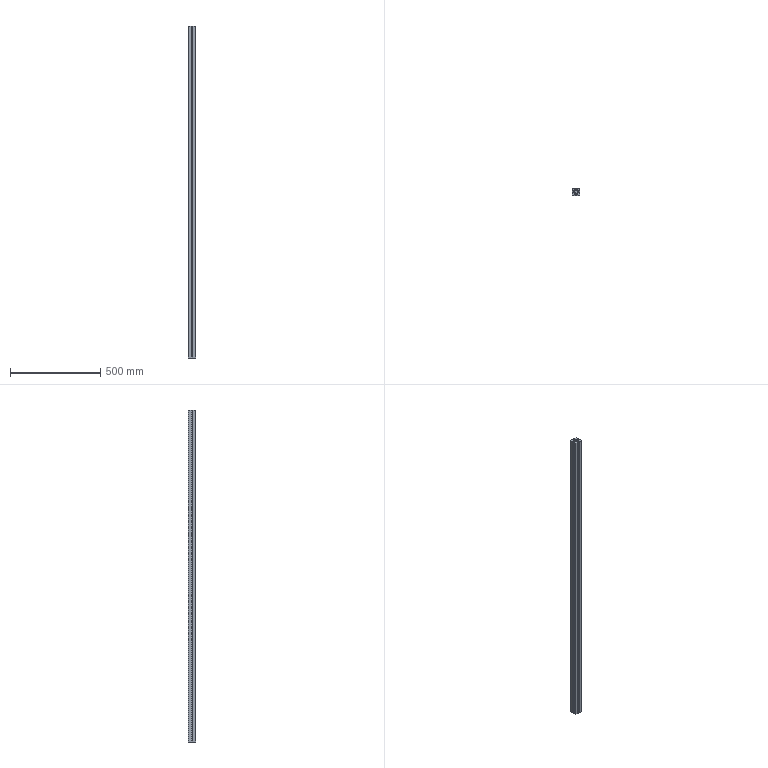Part | NX | 1 solid | 38 faces | box 40 x 40 x 1840 mm | volume 1840744 mm3 | plane 34 | cylinder 4 | commonest cylinder face diameters 19.333 x2 19.4 x2
STEP:
#1=CARTESIAN_POINT('',(-125.,655.75,0.));
#2=VERTEX_POINT('',#1);
#3=CARTESIAN_POINT('',(-121.5,655.75,0.));
#4=VERTEX_POINT('',#3);
#5=CARTESIAN_POINT('',(-125.,655.75,0.));
#6=DIRECTION('',(1.,0.,0.));
#7=VECTOR('',#6,1000.);
#8=LINE('',#5,#7);
#9=EDGE_CURVE('',#2,#4,#8,.T.);
#10=ORIENTED_EDGE('',*,*,#9,.T.);
#11=CARTESIAN_POINT('',(-121.5,655.75,-1840.));
#12=VERTEX_POINT('',#11);
#13=CARTESIAN_POINT('',(-121.5,655.75,-1840.));
#14=DIRECTION('',(0.,0.,1.));
#15=VECTOR('',#14,1000.);
#16=LINE('',#13,#15);
#17=EDGE_CURVE('',#12,#4,#16,.T.);
#18=ORIENTED_EDGE('',*,*,#17,.F.);
#19=CARTESIAN_POINT('',(-125.,655.75,-1840.));
#20=VERTEX_POINT('',#19);
#21=CARTESIAN_POINT('',(-125.,655.75,-1840.));
#22=DIRECTION('',(1.,0.,0.));
#23=VECTOR('',#22,1000.);
#24=LINE('',#21,#23);
#25=EDGE_CURVE('',#20,#12,#24,.T.);
#26=ORIENTED_EDGE('',*,*,#25,.F.);
#27=CARTESIAN_POINT('',(-125.,655.75,-1840.));
#28=DIRECTION('',(0.,0.,1.));
#29=VECTOR('',#28,1000.);
#30=LINE('',#27,#29);
#31=EDGE_CURVE('',#20,#2,#30,.T.);
#32=ORIENTED_EDGE('',*,*,#31,.T.);
#33=EDGE_LOOP('',(#10,#18,#26,#32));
#34=FACE_BOUND('',#33,.T.);
#35=CARTESIAN_POINT('',(-125.,655.75,-1840.));
#36=DIRECTION('',(0.,-1.,0.));
#37=DIRECTION('',(0.,0.,-1.));
#38=AXIS2_PLACEMENT_3D('',#35,#36,#37);
#39=PLANE('',#38);
#40=ADVANCED_FACE('',(#34),#39,.F.);
#41=CARTESIAN_POINT('',(-121.5,653.,0.));
#42=VERTEX_POINT('',#41);
#43=CARTESIAN_POINT('',(-121.5,655.75,0.));
#44=DIRECTION('',(0.,-1.,0.));
#45=VECTOR('',#44,1000.);
#46=LINE('',#43,#45);
#47=EDGE_CURVE('',#4,#42,#46,.T.);
#48=ORIENTED_EDGE('',*,*,#47,.T.);
#49=CARTESIAN_POINT('',(-121.5,653.,-1840.));
#50=VERTEX_POINT('',#49);
#51=CARTESIAN_POINT('',(-121.5,653.,-1840.));
#52=DIRECTION('',(0.,0.,1.));
#53=VECTOR('',#52,1000.);
#54=LINE('',#51,#53);
#55=EDGE_CURVE('',#50,#42,#54,.T.);
#56=ORIENTED_EDGE('',*,*,#55,.F.);
#57=CARTESIAN_POINT('',(-121.5,655.75,-1840.));
#58=DIRECTION('',(0.,-1.,0.));
#59=VECTOR('',#58,1000.);
#60=LINE('',#57,#59);
#61=EDGE_CURVE('',#12,#50,#60,.T.);
#62=ORIENTED_EDGE('',*,*,#61,.F.);
#63=ORIENTED_EDGE('',*,*,#17,.T.);
#64=EDGE_LOOP('',(#48,#56,#62,#63));
#65=FACE_BOUND('',#64,.T.);
#66=CARTESIAN_POINT('',(-121.5,655.75,-1840.));
#67=DIRECTION('',(-1.,0.,0.));
#68=DIRECTION('',(0.,0.,1.));
#69=AXIS2_PLACEMENT_3D('',#66,#67,#68);
#70=PLANE('',#69);
#71=ADVANCED_FACE('',(#65),#70,.F.);
#72=CARTESIAN_POINT('',(-114.5,653.,0.));
#73=VERTEX_POINT('',#72);
#74=CARTESIAN_POINT('',(-121.5,653.,0.));
#75=DIRECTION('',(1.,0.,0.));
#76=VECTOR('',#75,1000.);
#77=LINE('',#74,#76);
#78=EDGE_CURVE('',#42,#73,#77,.T.);
#79=ORIENTED_EDGE('',*,*,#78,.T.);
#80=CARTESIAN_POINT('',(-114.5,653.,-1840.));
#81=VERTEX_POINT('',#80);
#82=CARTESIAN_POINT('',(-114.5,653.,-1840.));
#83=DIRECTION('',(0.,0.,1.));
#84=VECTOR('',#83,1000.);
#85=LINE('',#82,#84);
#86=EDGE_CURVE('',#81,#73,#85,.T.);
#87=ORIENTED_EDGE('',*,*,#86,.F.);
#88=CARTESIAN_POINT('',(-121.5,653.,-1840.));
#89=DIRECTION('',(1.,0.,0.));
#90=VECTOR('',#89,1000.);
#91=LINE('',#88,#90);
#92=EDGE_CURVE('',#50,#81,#91,.T.);
#93=ORIENTED_EDGE('',*,*,#92,.F.);
#94=ORIENTED_EDGE('',*,*,#55,.T.);
#95=EDGE_LOOP('',(#79,#87,#93,#94));
#96=FACE_BOUND('',#95,.T.);
#97=CARTESIAN_POINT('',(-121.5,653.,-1840.));
#98=DIRECTION('',(0.,-1.,0.));
#99=DIRECTION('',(0.,0.,-1.));
#100=AXIS2_PLACEMENT_3D('',#97,#98,#99);
#101=PLANE('',#100);
#102=ADVANCED_FACE('',(#96),#101,.F.);
#103=CARTESIAN_POINT('',(-114.5,667.,0.));
#104=VERTEX_POINT('',#103);
#105=CARTESIAN_POINT('',(-121.167,660.,0.));
#106=DIRECTION('',(0.,0.,1.));
#107=DIRECTION('',(-1.,0.,0.));
#108=AXIS2_PLACEMENT_3D('',#105,#106,#107);
#109=CIRCLE('',#108,9.667);
#110=EDGE_CURVE('',#73,#104,#109,.T.);
#111=ORIENTED_EDGE('',*,*,#110,.T.);
#112=CARTESIAN_POINT('',(-114.5,667.,-1840.));
#113=VERTEX_POINT('',#112);
#114=CARTESIAN_POINT('',(-114.5,667.,-1840.));
#115=DIRECTION('',(0.,0.,1.));
#116=VECTOR('',#115,1000.);
#117=LINE('',#114,#116);
#118=EDGE_CURVE('',#113,#104,#117,.T.);
#119=ORIENTED_EDGE('',*,*,#118,.F.);
#120=CARTESIAN_POINT('',(-121.167,660.,-1840.));
#121=DIRECTION('',(0.,0.,1.));
#122=DIRECTION('',(-1.,0.,0.));
#123=AXIS2_PLACEMENT_3D('',#120,#121,#122);
#124=CIRCLE('',#123,9.667);
#125=EDGE_CURVE('',#81,#113,#124,.T.);
#126=ORIENTED_EDGE('',*,*,#125,.F.);
#127=ORIENTED_EDGE('',*,*,#86,.T.);
#128=EDGE_LOOP('',(#111,#119,#126,#127));
#129=FACE_BOUND('',#128,.T.);
#130=CARTESIAN_POINT('',(-121.167,660.,-1840.));
#131=DIRECTION('',(0.,0.,1.));
#132=DIRECTION('',(1.,0.,0.));
#133=AXIS2_PLACEMENT_3D('',#130,#131,#132);
#134=CYLINDRICAL_SURFACE('',#133,9.667);
#135=ADVANCED_FACE('',(#129),#134,.F.);
#136=CARTESIAN_POINT('',(-121.5,667.,0.));
#137=VERTEX_POINT('',#136);
#138=CARTESIAN_POINT('',(-114.5,667.,0.));
#139=DIRECTION('',(-1.,0.,0.));
#140=VECTOR('',#139,1000.);
#141=LINE('',#138,#140);
#142=EDGE_CURVE('',#104,#137,#141,.T.);
#143=ORIENTED_EDGE('',*,*,#142,.T.);
#144=CARTESIAN_POINT('',(-121.5,667.,-1840.));
#145=VERTEX_POINT('',#144);
#146=CARTESIAN_POINT('',(-121.5,667.,-1840.));
#147=DIRECTION('',(0.,0.,1.));
#148=VECTOR('',#147,1000.);
#149=LINE('',#146,#148);
#150=EDGE_CURVE('',#145,#137,#149,.T.);
#151=ORIENTED_EDGE('',*,*,#150,.F.);
#152=CARTESIAN_POINT('',(-114.5,667.,-1840.));
#153=DIRECTION('',(-1.,0.,0.));
#154=VECTOR('',#153,1000.);
#155=LINE('',#152,#154);
#156=EDGE_CURVE('',#113,#145,#155,.T.);
#157=ORIENTED_EDGE('',*,*,#156,.F.);
#158=ORIENTED_EDGE('',*,*,#118,.T.);
#159=EDGE_LOOP('',(#143,#151,#157,#158));
#160=FACE_BOUND('',#159,.T.);
#161=CARTESIAN_POINT('',(-114.5,667.,-1840.));
#162=DIRECTION('',(0.,1.,0.));
#163=DIRECTION('',(0.,0.,1.));
#164=AXIS2_PLACEMENT_3D('',#161,#162,#163);
#165=PLANE('',#164);
#166=ADVANCED_FACE('',(#160),#165,.F.);
#167=CARTESIAN_POINT('',(-121.5,664.25,0.));
#168=VERTEX_POINT('',#167);
#169=CARTESIAN_POINT('',(-121.5,667.,0.));
#170=DIRECTION('',(0.,-1.,0.));
#171=VECTOR('',#170,1000.);
#172=LINE('',#169,#171);
#173=EDGE_CURVE('',#137,#168,#172,.T.);
#174=ORIENTED_EDGE('',*,*,#173,.T.);
#175=CARTESIAN_POINT('',(-121.5,664.25,-1840.));
#176=VERTEX_POINT('',#175);
#177=CARTESIAN_POINT('',(-121.5,664.25,-1840.));
#178=DIRECTION('',(0.,0.,1.));
#179=VECTOR('',#178,1000.);
#180=LINE('',#177,#179);
#181=EDGE_CURVE('',#176,#168,#180,.T.);
#182=ORIENTED_EDGE('',*,*,#181,.F.);
#183=CARTESIAN_POINT('',(-121.5,667.,-1840.));
#184=DIRECTION('',(0.,-1.,0.));
#185=VECTOR('',#184,1000.);
#186=LINE('',#183,#185);
#187=EDGE_CURVE('',#145,#176,#186,.T.);
#188=ORIENTED_EDGE('',*,*,#187,.F.);
#189=ORIENTED_EDGE('',*,*,#150,.T.);
#190=EDGE_LOOP('',(#174,#182,#188,#189));
#191=FACE_BOUND('',#190,.T.);
#192=CARTESIAN_POINT('',(-121.5,667.,-1840.));
#193=DIRECTION('',(-1.,0.,0.));
#194=DIRECTION('',(0.,0.,1.));
#195=AXIS2_PLACEMENT_3D('',#192,#193,#194);
#196=PLANE('',#195);
#197=ADVANCED_FACE('',(#191),#196,.F.);
#198=CARTESIAN_POINT('',(-125.,664.25,0.));
#199=VERTEX_POINT('',#198);
#200=CARTESIAN_POINT('',(-121.5,664.25,0.));
#201=DIRECTION('',(-1.,0.,0.));
#202=VECTOR('',#201,1000.);
#203=LINE('',#200,#202);
#204=EDGE_CURVE('',#168,#199,#203,.T.);
#205=ORIENTED_EDGE('',*,*,#204,.T.);
#206=CARTESIAN_POINT('',(-125.,664.25,-1840.));
#207=VERTEX_POINT('',#206);
#208=CARTESIAN_POINT('',(-125.,664.25,-1840.));
#209=DIRECTION('',(0.,0.,1.));
#210=VECTOR('',#209,1000.);
#211=LINE('',#208,#210);
#212=EDGE_CURVE('',#207,#199,#211,.T.);
#213=ORIENTED_EDGE('',*,*,#212,.F.);
#214=CARTESIAN_POINT('',(-121.5,664.25,-1840.));
#215=DIRECTION('',(-1.,0.,0.));
#216=VECTOR('',#215,1000.);
#217=LINE('',#214,#216);
#218=EDGE_CURVE('',#176,#207,#217,.T.);
#219=ORIENTED_EDGE('',*,*,#218,.F.);
#220=ORIENTED_EDGE('',*,*,#181,.T.);
#221=EDGE_LOOP('',(#205,#213,#219,#220));
#222=FACE_BOUND('',#221,.T.);
#223=CARTESIAN_POINT('',(-121.5,664.25,-1840.));
#224=DIRECTION('',(0.,1.,0.));
#225=DIRECTION('',(0.,0.,1.));
#226=AXIS2_PLACEMENT_3D('',#223,#224,#225);
#227=PLANE('',#226);
#228=ADVANCED_FACE('',(#222),#227,.F.);
#229=CARTESIAN_POINT('',(-125.,680.,0.));
#230=VERTEX_POINT('',#229);
#231=CARTESIAN_POINT('',(-125.,680.,0.));
#232=DIRECTION('',(0.,1.,0.));
#233=VECTOR('',#232,1000.);
#234=LINE('',#231,#233);
#235=EDGE_CURVE('',#199,#230,#234,.T.);
#236=ORIENTED_EDGE('',*,*,#235,.T.);
#237=CARTESIAN_POINT('',(-125.,680.,-1840.));
#238=VERTEX_POINT('',#237);
#239=CARTESIAN_POINT('',(-125.,680.,-1840.));
#240=DIRECTION('',(0.,0.,1.));
#241=VECTOR('',#240,1000.);
#242=LINE('',#239,#241);
#243=EDGE_CURVE('',#238,#230,#242,.T.);
#244=ORIENTED_EDGE('',*,*,#243,.F.);
#245=CARTESIAN_POINT('',(-125.,664.25,-1840.));
#246=DIRECTION('',(0.,1.,0.));
#247=VECTOR('',#246,1000.);
#248=LINE('',#245,#247);
#249=EDGE_CURVE('',#207,#238,#248,.T.);
#250=ORIENTED_EDGE('',*,*,#249,.F.);
#251=ORIENTED_EDGE('',*,*,#212,.T.);
#252=EDGE_LOOP('',(#236,#244,#250,#251));
#253=FACE_BOUND('',#252,.T.);
#254=CARTESIAN_POINT('',(-125.,680.,-1840.));
#255=DIRECTION('',(1.,0.,0.));
#256=DIRECTION('',(0.,0.,-1.));
#257=AXIS2_PLACEMENT_3D('',#254,#255,#256);
#258=PLANE('',#257);
#259=ADVANCED_FACE('',(#253),#258,.F.);
#260=CARTESIAN_POINT('',(-109.25,680.,0.));
#261=VERTEX_POINT('',#260);
#262=CARTESIAN_POINT('',(-124.5,680.,0.));
#263=DIRECTION('',(1.,0.,0.));
#264=VECTOR('',#263,1000.);
#265=LINE('',#262,#264);
#266=EDGE_CURVE('',#230,#261,#265,.T.);
#267=ORIENTED_EDGE('',*,*,#266,.T.);
#268=CARTESIAN_POINT('',(-109.25,680.,-1840.));
#269=VERTEX_POINT('',#268);
#270=CARTESIAN_POINT('',(-109.25,680.,-1840.));
#271=DIRECTION('',(0.,0.,1.));
#272=VECTOR('',#271,1000.);
#273=LINE('',#270,#272);
#274=EDGE_CURVE('',#269,#261,#273,.T.);
#275=ORIENTED_EDGE('',*,*,#274,.F.);
#276=CARTESIAN_POINT('',(-124.5,680.,-1840.));
#277=DIRECTION('',(1.,0.,0.));
#278=VECTOR('',#277,1000.);
#279=LINE('',#276,#278);
#280=EDGE_CURVE('',#238,#269,#279,.T.);
#281=ORIENTED_EDGE('',*,*,#280,.F.);
#282=ORIENTED_EDGE('',*,*,#243,.T.);
#283=EDGE_LOOP('',(#267,#275,#281,#282));
#284=FACE_BOUND('',#283,.T.);
#285=CARTESIAN_POINT('',(-124.5,680.,-1840.));
#286=DIRECTION('',(0.,-1.,0.));
#287=DIRECTION('',(0.,0.,-1.));
#288=AXIS2_PLACEMENT_3D('',#285,#286,#287);
#289=PLANE('',#288);
#290=ADVANCED_FACE('',(#284),#289,.F.);
#291=CARTESIAN_POINT('',(-109.25,676.5,0.));
#292=VERTEX_POINT('',#291);
#293=CARTESIAN_POINT('',(-109.25,680.,0.));
#294=DIRECTION('',(0.,-1.,0.));
#295=VECTOR('',#294,1000.);
#296=LINE('',#293,#295);
#297=EDGE_CURVE('',#261,#292,#296,.T.);
#298=ORIENTED_EDGE('',*,*,#297,.T.);
#299=CARTESIAN_POINT('',(-109.25,676.5,-1840.));
#300=VERTEX_POINT('',#299);
#301=CARTESIAN_POINT('',(-109.25,676.5,-1840.));
#302=DIRECTION('',(0.,0.,1.));
#303=VECTOR('',#302,1000.);
#304=LINE('',#301,#303);
#305=EDGE_CURVE('',#300,#292,#304,.T.);
#306=ORIENTED_EDGE('',*,*,#305,.F.);
#307=CARTESIAN_POINT('',(-109.25,680.,-1840.));
#308=DIRECTION('',(0.,-1.,0.));
#309=VECTOR('',#308,1000.);
#310=LINE('',#307,#309);
#311=EDGE_CURVE('',#269,#300,#310,.T.);
#312=ORIENTED_EDGE('',*,*,#311,.F.);
#313=ORIENTED_EDGE('',*,*,#274,.T.);
#314=EDGE_LOOP('',(#298,#306,#312,#313));
#315=FACE_BOUND('',#314,.T.);
#316=CARTESIAN_POINT('',(-109.25,680.,-1840.));
#317=DIRECTION('',(-1.,0.,0.));
#318=DIRECTION('',(0.,0.,1.));
#319=AXIS2_PLACEMENT_3D('',#316,#317,#318);
#320=PLANE('',#319);
#321=ADVANCED_FACE('',(#315),#320,.F.);
#322=CARTESIAN_POINT('',(-111.5,676.5,0.));
#323=VERTEX_POINT('',#322);
#324=CARTESIAN_POINT('',(-109.25,676.5,0.));
#325=DIRECTION('',(-1.,0.,0.));
#326=VECTOR('',#325,1000.);
#327=LINE('',#324,#326);
#328=EDGE_CURVE('',#292,#323,#327,.T.);
#329=ORIENTED_EDGE('',*,*,#328,.T.);
#330=CARTESIAN_POINT('',(-111.5,676.5,-1840.));
#331=VERTEX_POINT('',#330);
#332=CARTESIAN_POINT('',(-111.5,676.5,-1840.));
#333=DIRECTION('',(0.,0.,1.));
#334=VECTOR('',#333,1000.);
#335=LINE('',#332,#334);
#336=EDGE_CURVE('',#331,#323,#335,.T.);
#337=ORIENTED_EDGE('',*,*,#336,.F.);
#338=CARTESIAN_POINT('',(-109.25,676.5,-1840.));
#339=DIRECTION('',(-1.,0.,0.));
#340=VECTOR('',#339,1000.);
#341=LINE('',#338,#340);
#342=EDGE_CURVE('',#300,#331,#341,.T.);
#343=ORIENTED_EDGE('',*,*,#342,.F.);
#344=ORIENTED_EDGE('',*,*,#305,.T.);
#345=EDGE_LOOP('',(#329,#337,#343,#344));
#346=FACE_BOUND('',#345,.T.);
#347=CARTESIAN_POINT('',(-109.25,676.5,-1840.));
#348=DIRECTION('',(0.,1.,0.));
#349=DIRECTION('',(0.,0.,1.));
#350=AXIS2_PLACEMENT_3D('',#347,#348,#349);
#351=PLANE('',#350);
#352=ADVANCED_FACE('',(#346),#351,.F.);
#353=CARTESIAN_POINT('',(-111.5,669.5,0.));
#354=VERTEX_POINT('',#353);
#355=CARTESIAN_POINT('',(-111.5,676.5,0.));
#356=DIRECTION('',(0.,-1.,0.));
#357=VECTOR('',#356,1000.);
#358=LINE('',#355,#357);
#359=EDGE_CURVE('',#323,#354,#358,.T.);
#360=ORIENTED_EDGE('',*,*,#359,.T.);
#361=CARTESIAN_POINT('',(-111.5,669.5,-1840.));
#362=VERTEX_POINT('',#361);
#363=CARTESIAN_POINT('',(-111.5,669.5,-1840.));
#364=DIRECTION('',(0.,0.,1.));
#365=VECTOR('',#364,1000.);
#366=LINE('',#363,#365);
#367=EDGE_CURVE('',#362,#354,#366,.T.);
#368=ORIENTED_EDGE('',*,*,#367,.F.);
#369=CARTESIAN_POINT('',(-111.5,676.5,-1840.));
#370=DIRECTION('',(0.,-1.,0.));
#371=VECTOR('',#370,1000.);
#372=LINE('',#369,#371);
#373=EDGE_CURVE('',#331,#362,#372,.T.);
#374=ORIENTED_EDGE('',*,*,#373,.F.);
#375=ORIENTED_EDGE('',*,*,#336,.T.);
#376=EDGE_LOOP('',(#360,#368,#374,#375));
#377=FACE_BOUND('',#376,.T.);
#378=CARTESIAN_POINT('',(-111.5,676.5,-1840.));
#379=DIRECTION('',(-1.,0.,0.));
#380=DIRECTION('',(0.,0.,1.));
#381=AXIS2_PLACEMENT_3D('',#378,#379,#380);
#382=PLANE('',#381);
#383=ADVANCED_FACE('',(#377),#382,.F.);
#384=CARTESIAN_POINT('',(-98.5,669.5,0.));
#385=VERTEX_POINT('',#384);
#386=CARTESIAN_POINT('',(-105.,676.7,0.));
#387=DIRECTION('',(0.,0.,1.));
#388=DIRECTION('',(-1.,0.,0.));
#389=AXIS2_PLACEMENT_3D('',#386,#387,#388);
#390=CIRCLE('',#389,9.7);
#391=EDGE_CURVE('',#354,#385,#390,.T.);
#392=ORIENTED_EDGE('',*,*,#391,.T.);
#393=CARTESIAN_POINT('',(-98.5,669.5,-1840.));
#394=VERTEX_POINT('',#393);
#395=CARTESIAN_POINT('',(-98.5,669.5,-1840.));
#396=DIRECTION('',(0.,0.,1.));
#397=VECTOR('',#396,1000.);
#398=LINE('',#395,#397);
#399=EDGE_CURVE('',#394,#385,#398,.T.);
#400=ORIENTED_EDGE('',*,*,#399,.F.);
#401=CARTESIAN_POINT('',(-105.,676.7,-1840.));
#402=DIRECTION('',(0.,0.,1.));
#403=DIRECTION('',(-1.,0.,0.));
#404=AXIS2_PLACEMENT_3D('',#401,#402,#403);
#405=CIRCLE('',#404,9.7);
#406=EDGE_CURVE('',#362,#394,#405,.T.);
#407=ORIENTED_EDGE('',*,*,#406,.F.);
#408=ORIENTED_EDGE('',*,*,#367,.T.);
#409=EDGE_LOOP('',(#392,#400,#407,#408));
#410=FACE_BOUND('',#409,.T.);
#411=CARTESIAN_POINT('',(-105.,676.7,-1840.));
#412=DIRECTION('',(0.,0.,1.));
#413=DIRECTION('',(1.,0.,0.));
#414=AXIS2_PLACEMENT_3D('',#411,#412,#413);
#415=CYLINDRICAL_SURFACE('',#414,9.7);
#416=ADVANCED_FACE('',(#410),#415,.F.);
#417=CARTESIAN_POINT('',(-98.5,676.5,0.));
#418=VERTEX_POINT('',#417);
#419=CARTESIAN_POINT('',(-98.5,669.5,0.));
#420=DIRECTION('',(0.,1.,0.));
#421=VECTOR('',#420,1000.);
#422=LINE('',#419,#421);
#423=EDGE_CURVE('',#385,#418,#422,.T.);
#424=ORIENTED_EDGE('',*,*,#423,.T.);
#425=CARTESIAN_POINT('',(-98.5,676.5,-1840.));
#426=VERTEX_POINT('',#425);
#427=CARTESIAN_POINT('',(-98.5,676.5,-1840.));
#428=DIRECTION('',(0.,0.,1.));
#429=VECTOR('',#428,1000.);
#430=LINE('',#427,#429);
#431=EDGE_CURVE('',#426,#418,#430,.T.);
#432=ORIENTED_EDGE('',*,*,#431,.F.);
#433=CARTESIAN_POINT('',(-98.5,669.5,-1840.));
#434=DIRECTION('',(0.,1.,0.));
#435=VECTOR('',#434,1000.);
#436=LINE('',#433,#435);
#437=EDGE_CURVE('',#394,#426,#436,.T.);
#438=ORIENTED_EDGE('',*,*,#437,.F.);
#439=ORIENTED_EDGE('',*,*,#399,.T.);
#440=EDGE_LOOP('',(#424,#432,#438,#439));
#441=FACE_BOUND('',#440,.T.);
#442=CARTESIAN_POINT('',(-98.5,669.5,-1840.));
#443=DIRECTION('',(1.,0.,0.));
#444=DIRECTION('',(0.,0.,-1.));
#445=AXIS2_PLACEMENT_3D('',#442,#443,#444);
#446=PLANE('',#445);
#447=ADVANCED_FACE('',(#441),#446,.F.);
#448=CARTESIAN_POINT('',(-100.75,676.5,0.));
#449=VERTEX_POINT('',#448);
#450=CARTESIAN_POINT('',(-98.5,676.5,0.));
#451=DIRECTION('',(-1.,0.,0.));
#452=VECTOR('',#451,1000.);
#453=LINE('',#450,#452);
#454=EDGE_CURVE('',#418,#449,#453,.T.);
#455=ORIENTED_EDGE('',*,*,#454,.T.);
#456=CARTESIAN_POINT('',(-100.75,676.5,-1840.));
#457=VERTEX_POINT('',#456);
#458=CARTESIAN_POINT('',(-100.75,676.5,-1840.));
#459=DIRECTION('',(0.,0.,1.));
#460=VECTOR('',#459,1000.);
#461=LINE('',#458,#460);
#462=EDGE_CURVE('',#457,#449,#461,.T.);
#463=ORIENTED_EDGE('',*,*,#462,.F.);
#464=CARTESIAN_POINT('',(-98.5,676.5,-1840.));
#465=DIRECTION('',(-1.,0.,0.));
#466=VECTOR('',#465,1000.);
#467=LINE('',#464,#466);
#468=EDGE_CURVE('',#426,#457,#467,.T.);
#469=ORIENTED_EDGE('',*,*,#468,.F.);
#470=ORIENTED_EDGE('',*,*,#431,.T.);
#471=EDGE_LOOP('',(#455,#463,#469,#470));
#472=FACE_BOUND('',#471,.T.);
#473=CARTESIAN_POINT('',(-98.5,676.5,-1840.));
#474=DIRECTION('',(0.,1.,0.));
#475=DIRECTION('',(0.,0.,1.));
#476=AXIS2_PLACEMENT_3D('',#473,#474,#475);
#477=PLANE('',#476);
#478=ADVANCED_FACE('',(#472),#477,.F.);
#479=CARTESIAN_POINT('',(-100.75,680.,0.));
#480=VERTEX_POINT('',#479);
#481=CARTESIAN_POINT('',(-100.75,676.5,0.));
#482=DIRECTION('',(0.,1.,0.));
#483=VECTOR('',#482,1000.);
#484=LINE('',#481,#483);
#485=EDGE_CURVE('',#449,#480,#484,.T.);
#486=ORIENTED_EDGE('',*,*,#485,.T.);
#487=CARTESIAN_POINT('',(-100.75,680.,-1840.));
#488=VERTEX_POINT('',#487);
#489=CARTESIAN_POINT('',(-100.75,680.,-1840.));
#490=DIRECTION('',(0.,0.,1.));
#491=VECTOR('',#490,1000.);
#492=LINE('',#489,#491);
#493=EDGE_CURVE('',#488,#480,#492,.T.);
#494=ORIENTED_EDGE('',*,*,#493,.F.);
#495=CARTESIAN_POINT('',(-100.75,676.5,-1840.));
#496=DIRECTION('',(0.,1.,0.));
#497=VECTOR('',#496,1000.);
#498=LINE('',#495,#497);
#499=EDGE_CURVE('',#457,#488,#498,.T.);
#500=ORIENTED_EDGE('',*,*,#499,.F.);
#501=ORIENTED_EDGE('',*,*,#462,.T.);
#502=EDGE_LOOP('',(#486,#494,#500,#501));
#503=FACE_BOUND('',#502,.T.);
#504=CARTESIAN_POINT('',(-100.75,676.5,-1840.));
#505=DIRECTION('',(1.,0.,0.));
#506=DIRECTION('',(0.,0.,-1.));
#507=AXIS2_PLACEMENT_3D('',#504,#505,#506);
#508=PLANE('',#507);
#509=ADVANCED_FACE('',(#503),#508,.F.);
#510=CARTESIAN_POINT('',(-85.,680.,0.));
#511=VERTEX_POINT('',#510);
#512=CARTESIAN_POINT('',(-85.5,680.,0.));
#513=DIRECTION('',(1.,0.,0.));
#514=VECTOR('',#513,1000.);
#515=LINE('',#512,#514);
#516=EDGE_CURVE('',#480,#511,#515,.T.);
#517=ORIENTED_EDGE('',*,*,#516,.T.);
#518=CARTESIAN_POINT('',(-85.,680.,-1840.));
#519=VERTEX_POINT('',#518);
#520=CARTESIAN_POINT('',(-85.,680.,-1840.));
#521=DIRECTION('',(0.,0.,1.));
#522=VECTOR('',#521,1000.);
#523=LINE('',#520,#522);
#524=EDGE_CURVE('',#519,#511,#523,.T.);
#525=ORIENTED_EDGE('',*,*,#524,.F.);
#526=CARTESIAN_POINT('',(-100.75,680.,-1840.));
#527=DIRECTION('',(1.,0.,0.));
#528=VECTOR('',#527,1000.);
#529=LINE('',#526,#528);
#530=EDGE_CURVE('',#488,#519,#529,.T.);
#531=ORIENTED_EDGE('',*,*,#530,.F.);
#532=ORIENTED_EDGE('',*,*,#493,.T.);
#533=EDGE_LOOP('',(#517,#525,#531,#532));
#534=FACE_BOUND('',#533,.T.);
#535=CARTESIAN_POINT('',(-85.5,680.,-1840.));
#536=DIRECTION('',(0.,-1.,0.));
#537=DIRECTION('',(0.,0.,-1.));
#538=AXIS2_PLACEMENT_3D('',#535,#536,#537);
#539=PLANE('',#538);
#540=ADVANCED_FACE('',(#534),#539,.F.);
#541=CARTESIAN_POINT('',(-85.,664.25,0.));
#542=VERTEX_POINT('',#541);
#543=CARTESIAN_POINT('',(-85.,679.5,0.));
#544=DIRECTION('',(0.,-1.,0.));
#545=VECTOR('',#544,1000.);
#546=LINE('',#543,#545);
#547=EDGE_CURVE('',#511,#542,#546,.T.);
#548=ORIENTED_EDGE('',*,*,#547,.T.);
#549=CARTESIAN_POINT('',(-85.,664.25,-1840.));
#550=VERTEX_POINT('',#549);
#551=CARTESIAN_POINT('',(-85.,664.25,-1840.));
#552=DIRECTION('',(0.,0.,1.));
#553=VECTOR('',#552,1000.);
#554=LINE('',#551,#553);
#555=EDGE_CURVE('',#550,#542,#554,.T.);
#556=ORIENTED_EDGE('',*,*,#555,.F.);
#557=CARTESIAN_POINT('',(-85.,680.,-1840.));
#558=DIRECTION('',(0.,-1.,0.));
#559=VECTOR('',#558,1000.);
#560=LINE('',#557,#559);
#561=EDGE_CURVE('',#519,#550,#560,.T.);
#562=ORIENTED_EDGE('',*,*,#561,.F.);
#563=ORIENTED_EDGE('',*,*,#524,.T.);
#564=EDGE_LOOP('',(#548,#556,#562,#563));
#565=FACE_BOUND('',#564,.T.);
#566=CARTESIAN_POINT('',(-85.,679.5,-1840.));
#567=DIRECTION('',(-1.,0.,0.));
#568=DIRECTION('',(0.,0.,1.));
#569=AXIS2_PLACEMENT_3D('',#566,#567,#568);
#570=PLANE('',#569);
#571=ADVANCED_FACE('',(#565),#570,.F.);
#572=CARTESIAN_POINT('',(-88.5,664.25,0.));
#573=VERTEX_POINT('',#572);
#574=CARTESIAN_POINT('',(-85.,664.25,0.));
#575=DIRECTION('',(-1.,0.,0.));
#576=VECTOR('',#575,1000.);
#577=LINE('',#574,#576);
#578=EDGE_CURVE('',#542,#573,#577,.T.);
#579=ORIENTED_EDGE('',*,*,#578,.T.);
#580=CARTESIAN_POINT('',(-88.5,664.25,-1840.));
#581=VERTEX_POINT('',#580);
#582=CARTESIAN_POINT('',(-88.5,664.25,-1840.));
#583=DIRECTION('',(0.,0.,1.));
#584=VECTOR('',#583,1000.);
#585=LINE('',#582,#584);
#586=EDGE_CURVE('',#581,#573,#585,.T.);
#587=ORIENTED_EDGE('',*,*,#586,.F.);
#588=CARTESIAN_POINT('',(-85.,664.25,-1840.));
#589=DIRECTION('',(-1.,0.,0.));
#590=VECTOR('',#589,1000.);
#591=LINE('',#588,#590);
#592=EDGE_CURVE('',#550,#581,#591,.T.);
#593=ORIENTED_EDGE('',*,*,#592,.F.);
#594=ORIENTED_EDGE('',*,*,#555,.T.);
#595=EDGE_LOOP('',(#579,#587,#593,#594));
#596=FACE_BOUND('',#595,.T.);
#597=CARTESIAN_POINT('',(-85.,664.25,-1840.));
#598=DIRECTION('',(0.,1.,0.));
#599=DIRECTION('',(0.,0.,1.));
#600=AXIS2_PLACEMENT_3D('',#597,#598,#599);
#601=PLANE('',#600);
#602=ADVANCED_FACE('',(#596),#601,.F.);
#603=CARTESIAN_POINT('',(-88.5,667.,0.));
#604=VERTEX_POINT('',#603);
#605=CARTESIAN_POINT('',(-88.5,664.25,0.));
#606=DIRECTION('',(0.,1.,0.));
#607=VECTOR('',#606,1000.);
#608=LINE('',#605,#607);
#609=EDGE_CURVE('',#573,#604,#608,.T.);
#610=ORIENTED_EDGE('',*,*,#609,.T.);
#611=CARTESIAN_POINT('',(-88.5,667.,-1840.));
#612=VERTEX_POINT('',#611);
#613=CARTESIAN_POINT('',(-88.5,667.,-1840.));
#614=DIRECTION('',(0.,0.,1.));
#615=VECTOR('',#614,1000.);
#616=LINE('',#613,#615);
#617=EDGE_CURVE('',#612,#604,#616,.T.);
#618=ORIENTED_EDGE('',*,*,#617,.F.);
#619=CARTESIAN_POINT('',(-88.5,664.25,-1840.));
#620=DIRECTION('',(0.,1.,0.));
#621=VECTOR('',#620,1000.);
#622=LINE('',#619,#621);
#623=EDGE_CURVE('',#581,#612,#622,.T.);
#624=ORIENTED_EDGE('',*,*,#623,.F.);
#625=ORIENTED_EDGE('',*,*,#586,.T.);
#626=EDGE_LOOP('',(#610,#618,#624,#625));
#627=FACE_BOUND('',#626,.T.);
#628=CARTESIAN_POINT('',(-88.5,664.25,-1840.));
#629=DIRECTION('',(1.,0.,0.));
#630=DIRECTION('',(0.,0.,-1.));
#631=AXIS2_PLACEMENT_3D('',#628,#629,#630);
#632=PLANE('',#631);
#633=ADVANCED_FACE('',(#627),#632,.F.);
#634=CARTESIAN_POINT('',(-95.5,667.,0.));
#635=VERTEX_POINT('',#634);
#636=CARTESIAN_POINT('',(-88.5,667.,0.));
#637=DIRECTION('',(-1.,0.,0.));
#638=VECTOR('',#637,1000.);
#639=LINE('',#636,#638);
#640=EDGE_CURVE('',#604,#635,#639,.T.);
#641=ORIENTED_EDGE('',*,*,#640,.T.);
#642=CARTESIAN_POINT('',(-95.5,667.,-1840.));
#643=VERTEX_POINT('',#642);
#644=CARTESIAN_POINT('',(-95.5,667.,-1840.));
#645=DIRECTION('',(0.,0.,1.));
#646=VECTOR('',#645,1000.);
#647=LINE('',#644,#646);
#648=EDGE_CURVE('',#643,#635,#647,.T.);
#649=ORIENTED_EDGE('',*,*,#648,.F.);
#650=CARTESIAN_POINT('',(-88.5,667.,-1840.));
#651=DIRECTION('',(-1.,0.,0.));
#652=VECTOR('',#651,1000.);
#653=LINE('',#650,#652);
#654=EDGE_CURVE('',#612,#643,#653,.T.);
#655=ORIENTED_EDGE('',*,*,#654,.F.);
#656=ORIENTED_EDGE('',*,*,#617,.T.);
#657=EDGE_LOOP('',(#641,#649,#655,#656));
#658=FACE_BOUND('',#657,.T.);
#659=CARTESIAN_POINT('',(-88.5,667.,-1840.));
#660=DIRECTION('',(0.,1.,0.));
#661=DIRECTION('',(0.,0.,1.));
#662=AXIS2_PLACEMENT_3D('',#659,#660,#661);
#663=PLANE('',#662);
#664=ADVANCED_FACE('',(#658),#663,.F.);
#665=CARTESIAN_POINT('',(-95.5,653.,0.));
#666=VERTEX_POINT('',#665);
#667=CARTESIAN_POINT('',(-88.833,660.,0.));
#668=DIRECTION('',(0.,0.,1.));
#669=DIRECTION('',(-1.,0.,0.));
#670=AXIS2_PLACEMENT_3D('',#667,#668,#669);
#671=CIRCLE('',#670,9.667);
#672=EDGE_CURVE('',#635,#666,#671,.T.);
#673=ORIENTED_EDGE('',*,*,#672,.T.);
#674=CARTESIAN_POINT('',(-95.5,653.,-1840.));
#675=VERTEX_POINT('',#674);
#676=CARTESIAN_POINT('',(-95.5,653.,-1840.));
#677=DIRECTION('',(0.,0.,1.));
#678=VECTOR('',#677,1000.);
#679=LINE('',#676,#678);
#680=EDGE_CURVE('',#675,#666,#679,.T.);
#681=ORIENTED_EDGE('',*,*,#680,.F.);
#682=CARTESIAN_POINT('',(-88.833,660.,-1840.));
#683=DIRECTION('',(0.,0.,1.));
#684=DIRECTION('',(-1.,0.,0.));
#685=AXIS2_PLACEMENT_3D('',#682,#683,#684);
#686=CIRCLE('',#685,9.667);
#687=EDGE_CURVE('',#643,#675,#686,.T.);
#688=ORIENTED_EDGE('',*,*,#687,.F.);
#689=ORIENTED_EDGE('',*,*,#648,.T.);
#690=EDGE_LOOP('',(#673,#681,#688,#689));
#691=FACE_BOUND('',#690,.T.);
#692=CARTESIAN_POINT('',(-88.833,660.,-1840.));
#693=DIRECTION('',(0.,0.,1.));
#694=DIRECTION('',(1.,0.,0.));
#695=AXIS2_PLACEMENT_3D('',#692,#693,#694);
#696=CYLINDRICAL_SURFACE('',#695,9.667);
#697=ADVANCED_FACE('',(#691),#696,.F.);
#698=CARTESIAN_POINT('',(-88.5,653.,0.));
#699=VERTEX_POINT('',#698);
#700=CARTESIAN_POINT('',(-95.5,653.,0.));
#701=DIRECTION('',(1.,0.,0.));
#702=VECTOR('',#701,1000.);
#703=LINE('',#700,#702);
#704=EDGE_CURVE('',#666,#699,#703,.T.);
#705=ORIENTED_EDGE('',*,*,#704,.T.);
#706=CARTESIAN_POINT('',(-88.5,653.,-1840.));
#707=VERTEX_POINT('',#706);
#708=CARTESIAN_POINT('',(-88.5,653.,-1840.));
#709=DIRECTION('',(0.,0.,1.));
#710=VECTOR('',#709,1000.);
#711=LINE('',#708,#710);
#712=EDGE_CURVE('',#707,#699,#711,.T.);
#713=ORIENTED_EDGE('',*,*,#712,.F.);
#714=CARTESIAN_POINT('',(-95.5,653.,-1840.));
#715=DIRECTION('',(1.,0.,0.));
#716=VECTOR('',#715,1000.);
#717=LINE('',#714,#716);
#718=EDGE_CURVE('',#675,#707,#717,.T.);
#719=ORIENTED_EDGE('',*,*,#718,.F.);
#720=ORIENTED_EDGE('',*,*,#680,.T.);
#721=EDGE_LOOP('',(#705,#713,#719,#720));
#722=FACE_BOUND('',#721,.T.);
#723=CARTESIAN_POINT('',(-95.5,653.,-1840.));
#724=DIRECTION('',(0.,-1.,0.));
#725=DIRECTION('',(0.,0.,-1.));
#726=AXIS2_PLACEMENT_3D('',#723,#724,#725);
#727=PLANE('',#726);
#728=ADVANCED_FACE('',(#722),#727,.F.);
#729=CARTESIAN_POINT('',(-88.5,655.75,0.));
#730=VERTEX_POINT('',#729);
#731=CARTESIAN_POINT('',(-88.5,653.,0.));
#732=DIRECTION('',(0.,1.,0.));
#733=VECTOR('',#732,1000.);
#734=LINE('',#731,#733);
#735=EDGE_CURVE('',#699,#730,#734,.T.);
#736=ORIENTED_EDGE('',*,*,#735,.T.);
#737=CARTESIAN_POINT('',(-88.5,655.75,-1840.));
#738=VERTEX_POINT('',#737);
#739=CARTESIAN_POINT('',(-88.5,655.75,-1840.));
#740=DIRECTION('',(0.,0.,1.));
#741=VECTOR('',#740,1000.);
#742=LINE('',#739,#741);
#743=EDGE_CURVE('',#738,#730,#742,.T.);
#744=ORIENTED_EDGE('',*,*,#743,.F.);
#745=CARTESIAN_POINT('',(-88.5,653.,-1840.));
#746=DIRECTION('',(0.,1.,0.));
#747=VECTOR('',#746,1000.);
#748=LINE('',#745,#747);
#749=EDGE_CURVE('',#707,#738,#748,.T.);
#750=ORIENTED_EDGE('',*,*,#749,.F.);
#751=ORIENTED_EDGE('',*,*,#712,.T.);
#752=EDGE_LOOP('',(#736,#744,#750,#751));
#753=FACE_BOUND('',#752,.T.);
#754=CARTESIAN_POINT('',(-88.5,653.,-1840.));
#755=DIRECTION('',(1.,0.,0.));
#756=DIRECTION('',(0.,0.,-1.));
#757=AXIS2_PLACEMENT_3D('',#754,#755,#756);
#758=PLANE('',#757);
#759=ADVANCED_FACE('',(#753),#758,.F.);
#760=CARTESIAN_POINT('',(-85.,655.75,0.));
#761=VERTEX_POINT('',#760);
#762=CARTESIAN_POINT('',(-88.5,655.75,0.));
#763=DIRECTION('',(1.,0.,0.));
#764=VECTOR('',#763,1000.);
#765=LINE('',#762,#764);
#766=EDGE_CURVE('',#730,#761,#765,.T.);
#767=ORIENTED_EDGE('',*,*,#766,.T.);
#768=CARTESIAN_POINT('',(-85.,655.75,-1840.));
#769=VERTEX_POINT('',#768);
#770=CARTESIAN_POINT('',(-85.,655.75,-1840.));
#771=DIRECTION('',(0.,0.,1.));
#772=VECTOR('',#771,1000.);
#773=LINE('',#770,#772);
#774=EDGE_CURVE('',#769,#761,#773,.T.);
#775=ORIENTED_EDGE('',*,*,#774,.F.);
#776=CARTESIAN_POINT('',(-88.5,655.75,-1840.));
#777=DIRECTION('',(1.,0.,0.));
#778=VECTOR('',#777,1000.);
#779=LINE('',#776,#778);
#780=EDGE_CURVE('',#738,#769,#779,.T.);
#781=ORIENTED_EDGE('',*,*,#780,.F.);
#782=ORIENTED_EDGE('',*,*,#743,.T.);
#783=EDGE_LOOP('',(#767,#775,#781,#782));
#784=FACE_BOUND('',#783,.T.);
#785=CARTESIAN_POINT('',(-88.5,655.75,-1840.));
#786=DIRECTION('',(0.,-1.,0.));
#787=DIRECTION('',(0.,0.,-1.));
#788=AXIS2_PLACEMENT_3D('',#785,#786,#787);
#789=PLANE('',#788);
#790=ADVANCED_FACE('',(#784),#789,.F.);
#791=CARTESIAN_POINT('',(-85.,640.,0.));
#792=VERTEX_POINT('',#791);
#793=CARTESIAN_POINT('',(-85.,640.5,0.));
#794=DIRECTION('',(0.,-1.,0.));
#795=VECTOR('',#794,1000.);
#796=LINE('',#793,#795);
#797=EDGE_CURVE('',#761,#792,#796,.T.);
#798=ORIENTED_EDGE('',*,*,#797,.T.);
#799=CARTESIAN_POINT('',(-85.,640.,-1840.));
#800=VERTEX_POINT('',#799);
#801=CARTESIAN_POINT('',(-85.,640.,-1840.));
#802=DIRECTION('',(0.,0.,1.));
#803=VECTOR('',#802,1000.);
#804=LINE('',#801,#803);
#805=EDGE_CURVE('',#800,#792,#804,.T.);
#806=ORIENTED_EDGE('',*,*,#805,.F.);
#807=CARTESIAN_POINT('',(-85.,655.75,-1840.));
#808=DIRECTION('',(0.,-1.,0.));
#809=VECTOR('',#808,1000.);
#810=LINE('',#807,#809);
#811=EDGE_CURVE('',#769,#800,#810,.T.);
#812=ORIENTED_EDGE('',*,*,#811,.F.);
#813=ORIENTED_EDGE('',*,*,#774,.T.);
#814=EDGE_LOOP('',(#798,#806,#812,#813));
#815=FACE_BOUND('',#814,.T.);
#816=CARTESIAN_POINT('',(-85.,640.5,-1840.));
#817=DIRECTION('',(-1.,0.,0.));
#818=DIRECTION('',(0.,0.,1.));
#819=AXIS2_PLACEMENT_3D('',#816,#817,#818);
#820=PLANE('',#819);
#821=ADVANCED_FACE('',(#815),#820,.F.);
#822=CARTESIAN_POINT('',(-100.75,640.,0.));
#823=VERTEX_POINT('',#822);
#824=CARTESIAN_POINT('',(-85.5,640.,0.));
#825=DIRECTION('',(-1.,0.,0.));
#826=VECTOR('',#825,1000.);
#827=LINE('',#824,#826);
#828=EDGE_CURVE('',#792,#823,#827,.T.);
#829=ORIENTED_EDGE('',*,*,#828,.T.);
#830=CARTESIAN_POINT('',(-100.75,640.,-1840.));
#831=VERTEX_POINT('',#830);
#832=CARTESIAN_POINT('',(-100.75,640.,-1840.));
#833=DIRECTION('',(0.,0.,1.));
#834=VECTOR('',#833,1000.);
#835=LINE('',#832,#834);
#836=EDGE_CURVE('',#831,#823,#835,.T.);
#837=ORIENTED_EDGE('',*,*,#836,.F.);
#838=CARTESIAN_POINT('',(-85.,640.,-1840.));
#839=DIRECTION('',(-1.,0.,0.));
#840=VECTOR('',#839,1000.);
#841=LINE('',#838,#840);
#842=EDGE_CURVE('',#800,#831,#841,.T.);
#843=ORIENTED_EDGE('',*,*,#842,.F.);
#844=ORIENTED_EDGE('',*,*,#805,.T.);
#845=EDGE_LOOP('',(#829,#837,#843,#844));
#846=FACE_BOUND('',#845,.T.);
#847=CARTESIAN_POINT('',(-85.5,640.,-1840.));
#848=DIRECTION('',(0.,1.,0.));
#849=DIRECTION('',(-1.,0.,0.));
#850=AXIS2_PLACEMENT_3D('',#847,#848,#849);
#851=PLANE('',#850);
#852=ADVANCED_FACE('',(#846),#851,.F.);
#853=CARTESIAN_POINT('',(-100.75,643.5,0.));
#854=VERTEX_POINT('',#853);
#855=CARTESIAN_POINT('',(-100.75,640.,0.));
#856=DIRECTION('',(0.,1.,0.));
#857=VECTOR('',#856,1000.);
#858=LINE('',#855,#857);
#859=EDGE_CURVE('',#823,#854,#858,.T.);
#860=ORIENTED_EDGE('',*,*,#859,.T.);
#861=CARTESIAN_POINT('',(-100.75,643.5,-1840.));
#862=VERTEX_POINT('',#861);
#863=CARTESIAN_POINT('',(-100.75,643.5,-1840.));
#864=DIRECTION('',(0.,0.,1.));
#865=VECTOR('',#864,1000.);
#866=LINE('',#863,#865);
#867=EDGE_CURVE('',#862,#854,#866,.T.);
#868=ORIENTED_EDGE('',*,*,#867,.F.);
#869=CARTESIAN_POINT('',(-100.75,640.,-1840.));
#870=DIRECTION('',(0.,1.,0.));
#871=VECTOR('',#870,1000.);
#872=LINE('',#869,#871);
#873=EDGE_CURVE('',#831,#862,#872,.T.);
#874=ORIENTED_EDGE('',*,*,#873,.F.);
#875=ORIENTED_EDGE('',*,*,#836,.T.);
#876=EDGE_LOOP('',(#860,#868,#874,#875));
#877=FACE_BOUND('',#876,.T.);
#878=CARTESIAN_POINT('',(-100.75,640.,-1840.));
#879=DIRECTION('',(1.,0.,0.));
#880=DIRECTION('',(0.,0.,-1.));
#881=AXIS2_PLACEMENT_3D('',#878,#879,#880);
#882=PLANE('',#881);
#883=ADVANCED_FACE('',(#877),#882,.F.);
#884=CARTESIAN_POINT('',(-98.5,643.5,0.));
#885=VERTEX_POINT('',#884);
#886=CARTESIAN_POINT('',(-100.75,643.5,0.));
#887=DIRECTION('',(1.,0.,0.));
#888=VECTOR('',#887,1000.);
#889=LINE('',#886,#888);
#890=EDGE_CURVE('',#854,#885,#889,.T.);
#891=ORIENTED_EDGE('',*,*,#890,.T.);
#892=CARTESIAN_POINT('',(-98.5,643.5,-1840.));
#893=VERTEX_POINT('',#892);
#894=CARTESIAN_POINT('',(-98.5,643.5,-1840.));
#895=DIRECTION('',(0.,0.,1.));
#896=VECTOR('',#895,1000.);
#897=LINE('',#894,#896);
#898=EDGE_CURVE('',#893,#885,#897,.T.);
#899=ORIENTED_EDGE('',*,*,#898,.F.);
#900=CARTESIAN_POINT('',(-100.75,643.5,-1840.));
#901=DIRECTION('',(1.,0.,0.));
#902=VECTOR('',#901,1000.);
#903=LINE('',#900,#902);
#904=EDGE_CURVE('',#862,#893,#903,.T.);
#905=ORIENTED_EDGE('',*,*,#904,.F.);
#906=ORIENTED_EDGE('',*,*,#867,.T.);
#907=EDGE_LOOP('',(#891,#899,#905,#906));
#908=FACE_BOUND('',#907,.T.);
#909=CARTESIAN_POINT('',(-100.75,643.5,-1840.));
#910=DIRECTION('',(0.,-1.,0.));
#911=DIRECTION('',(0.,0.,-1.));
#912=AXIS2_PLACEMENT_3D('',#909,#910,#911);
#913=PLANE('',#912);
#914=ADVANCED_FACE('',(#908),#913,.F.);
#915=CARTESIAN_POINT('',(-98.5,650.5,0.));
#916=VERTEX_POINT('',#915);
#917=CARTESIAN_POINT('',(-98.5,643.5,0.));
#918=DIRECTION('',(0.,1.,0.));
#919=VECTOR('',#918,1000.);
#920=LINE('',#917,#919);
#921=EDGE_CURVE('',#885,#916,#920,.T.);
#922=ORIENTED_EDGE('',*,*,#921,.T.);
#923=CARTESIAN_POINT('',(-98.5,650.5,-1840.));
#924=VERTEX_POINT('',#923);
#925=CARTESIAN_POINT('',(-98.5,650.5,-1840.));
#926=DIRECTION('',(0.,0.,1.));
#927=VECTOR('',#926,1000.);
#928=LINE('',#925,#927);
#929=EDGE_CURVE('',#924,#916,#928,.T.);
#930=ORIENTED_EDGE('',*,*,#929,.F.);
#931=CARTESIAN_POINT('',(-98.5,643.5,-1840.));
#932=DIRECTION('',(0.,1.,0.));
#933=VECTOR('',#932,1000.);
#934=LINE('',#931,#933);
#935=EDGE_CURVE('',#893,#924,#934,.T.);
#936=ORIENTED_EDGE('',*,*,#935,.F.);
#937=ORIENTED_EDGE('',*,*,#898,.T.);
#938=EDGE_LOOP('',(#922,#930,#936,#937));
#939=FACE_BOUND('',#938,.T.);
#940=CARTESIAN_POINT('',(-98.5,643.5,-1840.));
#941=DIRECTION('',(1.,0.,0.));
#942=DIRECTION('',(0.,1.,0.));
#943=AXIS2_PLACEMENT_3D('',#940,#941,#942);
#944=PLANE('',#943);
#945=ADVANCED_FACE('',(#939),#944,.F.);
#946=CARTESIAN_POINT('',(-111.5,650.5,0.));
#947=VERTEX_POINT('',#946);
#948=CARTESIAN_POINT('',(-105.,643.3,0.));
#949=DIRECTION('',(0.,0.,1.));
#950=DIRECTION('',(-1.,0.,0.));
#951=AXIS2_PLACEMENT_3D('',#948,#949,#950);
#952=CIRCLE('',#951,9.7);
#953=EDGE_CURVE('',#916,#947,#952,.T.);
#954=ORIENTED_EDGE('',*,*,#953,.T.);
#955=CARTESIAN_POINT('',(-111.5,650.5,-1840.));
#956=VERTEX_POINT('',#955);
#957=CARTESIAN_POINT('',(-111.5,650.5,-1840.));
#958=DIRECTION('',(0.,0.,1.));
#959=VECTOR('',#958,1000.);
#960=LINE('',#957,#959);
#961=EDGE_CURVE('',#956,#947,#960,.T.);
#962=ORIENTED_EDGE('',*,*,#961,.F.);
#963=CARTESIAN_POINT('',(-105.,643.3,-1840.));
#964=DIRECTION('',(0.,0.,1.));
#965=DIRECTION('',(-1.,0.,0.));
#966=AXIS2_PLACEMENT_3D('',#963,#964,#965);
#967=CIRCLE('',#966,9.7);
#968=EDGE_CURVE('',#924,#956,#967,.T.);
#969=ORIENTED_EDGE('',*,*,#968,.F.);
#970=ORIENTED_EDGE('',*,*,#929,.T.);
#971=EDGE_LOOP('',(#954,#962,#969,#970));
#972=FACE_BOUND('',#971,.T.);
#973=CARTESIAN_POINT('',(-105.,643.3,-1840.));
#974=DIRECTION('',(0.,0.,1.));
#975=DIRECTION('',(1.,0.,0.));
#976=AXIS2_PLACEMENT_3D('',#973,#974,#975);
#977=CYLINDRICAL_SURFACE('',#976,9.7);
#978=ADVANCED_FACE('',(#972),#977,.F.);
#979=CARTESIAN_POINT('',(-111.5,643.5,0.));
#980=VERTEX_POINT('',#979);
#981=CARTESIAN_POINT('',(-111.5,650.5,0.));
#982=DIRECTION('',(0.,-1.,0.));
#983=VECTOR('',#982,1000.);
#984=LINE('',#981,#983);
#985=EDGE_CURVE('',#947,#980,#984,.T.);
#986=ORIENTED_EDGE('',*,*,#985,.T.);
#987=CARTESIAN_POINT('',(-111.5,643.5,-1840.));
#988=VERTEX_POINT('',#987);
#989=CARTESIAN_POINT('',(-111.5,643.5,-1840.));
#990=DIRECTION('',(0.,0.,1.));
#991=VECTOR('',#990,1000.);
#992=LINE('',#989,#991);
#993=EDGE_CURVE('',#988,#980,#992,.T.);
#994=ORIENTED_EDGE('',*,*,#993,.F.);
#995=CARTESIAN_POINT('',(-111.5,650.5,-1840.));
#996=DIRECTION('',(0.,-1.,0.));
#997=VECTOR('',#996,1000.);
#998=LINE('',#995,#997);
#999=EDGE_CURVE('',#956,#988,#998,.T.);
#1000=ORIENTED_EDGE('',*,*,#999,.F.);
#1001=ORIENTED_EDGE('',*,*,#961,.T.);
#1002=EDGE_LOOP('',(#986,#994,#1000,#1001));
#1003=FACE_BOUND('',#1002,.T.);
#1004=CARTESIAN_POINT('',(-111.5,650.5,-1840.));
#1005=DIRECTION('',(-1.,0.,0.));
#1006=DIRECTION('',(0.,-1.,0.));
#1007=AXIS2_PLACEMENT_3D('',#1004,#1005,#1006);
#1008=PLANE('',#1007);
#1009=ADVANCED_FACE('',(#1003),#1008,.F.);
#1010=CARTESIAN_POINT('',(-109.25,643.5,0.));
#1011=VERTEX_POINT('',#1010);
#1012=CARTESIAN_POINT('',(-111.5,643.5,0.));
#1013=DIRECTION('',(1.,0.,0.));
#1014=VECTOR('',#1013,1000.);
#1015=LINE('',#1012,#1014);
#1016=EDGE_CURVE('',#980,#1011,#1015,.T.);
#1017=ORIENTED_EDGE('',*,*,#1016,.T.);
#1018=CARTESIAN_POINT('',(-109.25,643.5,-1840.));
#1019=VERTEX_POINT('',#1018);
#1020=CARTESIAN_POINT('',(-109.25,643.5,-1840.));
#1021=DIRECTION('',(0.,0.,1.));
#1022=VECTOR('',#1021,1000.);
#1023=LINE('',#1020,#1022);
#1024=EDGE_CURVE('',#1019,#1011,#1023,.T.);
#1025=ORIENTED_EDGE('',*,*,#1024,.F.);
#1026=CARTESIAN_POINT('',(-111.5,643.5,-1840.));
#1027=DIRECTION('',(1.,0.,0.));
#1028=VECTOR('',#1027,1000.);
#1029=LINE('',#1026,#1028);
#1030=EDGE_CURVE('',#988,#1019,#1029,.T.);
#1031=ORIENTED_EDGE('',*,*,#1030,.F.);
#1032=ORIENTED_EDGE('',*,*,#993,.T.);
#1033=EDGE_LOOP('',(#1017,#1025,#1031,#1032));
#1034=FACE_BOUND('',#1033,.T.);
#1035=CARTESIAN_POINT('',(-111.5,643.5,-1840.));
#1036=DIRECTION('',(0.,-1.,0.));
#1037=DIRECTION('',(0.,0.,-1.));
#1038=AXIS2_PLACEMENT_3D('',#1035,#1036,#1037);
#1039=PLANE('',#1038);
#1040=ADVANCED_FACE('',(#1034),#1039,.F.);
#1041=CARTESIAN_POINT('',(-109.25,640.,0.));
#1042=VERTEX_POINT('',#1041);
#1043=CARTESIAN_POINT('',(-109.25,643.5,0.));
#1044=DIRECTION('',(0.,-1.,0.));
#1045=VECTOR('',#1044,1000.);
#1046=LINE('',#1043,#1045);
#1047=EDGE_CURVE('',#1011,#1042,#1046,.T.);
#1048=ORIENTED_EDGE('',*,*,#1047,.T.);
#1049=CARTESIAN_POINT('',(-109.25,640.,-1840.));
#1050=VERTEX_POINT('',#1049);
#1051=CARTESIAN_POINT('',(-109.25,640.,-1840.));
#1052=DIRECTION('',(0.,0.,1.));
#1053=VECTOR('',#1052,1000.);
#1054=LINE('',#1051,#1053);
#1055=EDGE_CURVE('',#1050,#1042,#1054,.T.);
#1056=ORIENTED_EDGE('',*,*,#1055,.F.);
#1057=CARTESIAN_POINT('',(-109.25,643.5,-1840.));
#1058=DIRECTION('',(0.,-1.,0.));
#1059=VECTOR('',#1058,1000.);
#1060=LINE('',#1057,#1059);
#1061=EDGE_CURVE('',#1019,#1050,#1060,.T.);
#1062=ORIENTED_EDGE('',*,*,#1061,.F.);
#1063=ORIENTED_EDGE('',*,*,#1024,.T.);
#1064=EDGE_LOOP('',(#1048,#1056,#1062,#1063));
#1065=FACE_BOUND('',#1064,.T.);
#1066=CARTESIAN_POINT('',(-109.25,643.5,-1840.));
#1067=DIRECTION('',(-1.,0.,0.));
#1068=DIRECTION('',(0.,0.,1.));
#1069=AXIS2_PLACEMENT_3D('',#1066,#1067,#1068);
#1070=PLANE('',#1069);
#1071=ADVANCED_FACE('',(#1065),#1070,.F.);
#1072=CARTESIAN_POINT('',(-125.,640.,0.));
#1073=VERTEX_POINT('',#1072);
#1074=CARTESIAN_POINT('',(-125.,640.,0.));
#1075=DIRECTION('',(-1.,0.,0.));
#1076=VECTOR('',#1075,1000.);
#1077=LINE('',#1074,#1076);
#1078=EDGE_CURVE('',#1042,#1073,#1077,.T.);
#1079=ORIENTED_EDGE('',*,*,#1078,.T.);
#1080=CARTESIAN_POINT('',(-125.,640.,-1840.));
#1081=VERTEX_POINT('',#1080);
#1082=CARTESIAN_POINT('',(-125.,640.,-1840.));
#1083=DIRECTION('',(0.,0.,1.));
#1084=VECTOR('',#1083,1000.);
#1085=LINE('',#1082,#1084);
#1086=EDGE_CURVE('',#1081,#1073,#1085,.T.);
#1087=ORIENTED_EDGE('',*,*,#1086,.F.);
#1088=CARTESIAN_POINT('',(-109.25,640.,-1840.));
#1089=DIRECTION('',(-1.,0.,0.));
#1090=VECTOR('',#1089,1000.);
#1091=LINE('',#1088,#1090);
#1092=EDGE_CURVE('',#1050,#1081,#1091,.T.);
#1093=ORIENTED_EDGE('',*,*,#1092,.F.);
#1094=ORIENTED_EDGE('',*,*,#1055,.T.);
#1095=EDGE_LOOP('',(#1079,#1087,#1093,#1094));
#1096=FACE_BOUND('',#1095,.T.);
#1097=CARTESIAN_POINT('',(-125.,640.,-1840.));
#1098=DIRECTION('',(0.,1.,0.));
#1099=DIRECTION('',(0.,0.,1.));
#1100=AXIS2_PLACEMENT_3D('',#1097,#1098,#1099);
#1101=PLANE('',#1100);
#1102=ADVANCED_FACE('',(#1096),#1101,.F.);
#1103=CARTESIAN_POINT('',(-125.,640.5,0.));
#1104=DIRECTION('',(0.,1.,0.));
#1105=VECTOR('',#1104,1000.);
#1106=LINE('',#1103,#1105);
#1107=EDGE_CURVE('',#1073,#2,#1106,.T.);
#1108=ORIENTED_EDGE('',*,*,#1107,.T.);
#1109=ORIENTED_EDGE('',*,*,#31,.F.);
#1110=CARTESIAN_POINT('',(-125.,640.5,-1840.));
#1111=DIRECTION('',(0.,1.,0.));
#1112=VECTOR('',#1111,1000.);
#1113=LINE('',#1110,#1112);
#1114=EDGE_CURVE('',#1081,#20,#1113,.T.);
#1115=ORIENTED_EDGE('',*,*,#1114,.F.);
#1116=ORIENTED_EDGE('',*,*,#1086,.T.);
#1117=EDGE_LOOP('',(#1108,#1109,#1115,#1116));
#1118=FACE_BOUND('',#1117,.T.);
#1119=CARTESIAN_POINT('',(-125.,640.5,-1840.));
#1120=DIRECTION('',(1.,0.,0.));
#1121=DIRECTION('',(0.,0.,-1.));
#1122=AXIS2_PLACEMENT_3D('',#1119,#1120,#1121);
#1123=PLANE('',#1122);
#1124=ADVANCED_FACE('',(#1118),#1123,.F.);
#1125=ORIENTED_EDGE('',*,*,#1114,.T.);
#1126=ORIENTED_EDGE('',*,*,#25,.T.);
#1127=ORIENTED_EDGE('',*,*,#61,.T.);
#1128=ORIENTED_EDGE('',*,*,#92,.T.);
#1129=ORIENTED_EDGE('',*,*,#125,.T.);
#1130=ORIENTED_EDGE('',*,*,#156,.T.);
#1131=ORIENTED_EDGE('',*,*,#187,.T.);
#1132=ORIENTED_EDGE('',*,*,#218,.T.);
#1133=ORIENTED_EDGE('',*,*,#249,.T.);
#1134=ORIENTED_EDGE('',*,*,#280,.T.);
#1135=ORIENTED_EDGE('',*,*,#311,.T.);
#1136=ORIENTED_EDGE('',*,*,#342,.T.);
#1137=ORIENTED_EDGE('',*,*,#373,.T.);
#1138=ORIENTED_EDGE('',*,*,#406,.T.);
#1139=ORIENTED_EDGE('',*,*,#437,.T.);
#1140=ORIENTED_EDGE('',*,*,#468,.T.);
#1141=ORIENTED_EDGE('',*,*,#499,.T.);
#1142=ORIENTED_EDGE('',*,*,#530,.T.);
#1143=ORIENTED_EDGE('',*,*,#561,.T.);
#1144=ORIENTED_EDGE('',*,*,#592,.T.);
#1145=ORIENTED_EDGE('',*,*,#623,.T.);
#1146=ORIENTED_EDGE('',*,*,#654,.T.);
#1147=ORIENTED_EDGE('',*,*,#687,.T.);
#1148=ORIENTED_EDGE('',*,*,#718,.T.);
#1149=ORIENTED_EDGE('',*,*,#749,.T.);
#1150=ORIENTED_EDGE('',*,*,#780,.T.);
#1151=ORIENTED_EDGE('',*,*,#811,.T.);
#1152=ORIENTED_EDGE('',*,*,#842,.T.);
#1153=ORIENTED_EDGE('',*,*,#873,.T.);
#1154=ORIENTED_EDGE('',*,*,#904,.T.);
#1155=ORIENTED_EDGE('',*,*,#935,.T.);
#1156=ORIENTED_EDGE('',*,*,#968,.T.);
#1157=ORIENTED_EDGE('',*,*,#999,.T.);
#1158=ORIENTED_EDGE('',*,*,#1030,.T.);
#1159=ORIENTED_EDGE('',*,*,#1061,.T.);
#1160=ORIENTED_EDGE('',*,*,#1092,.T.);
#1161=EDGE_LOOP('',(#1125,#1126,#1127,#1128,#1129,#1130,#1131,#1132,#1133,#1134,#1135,#1136,#1137,#1138,#1139,#1140,#1141,#1142,#1143,#1144,#1145,#1146,#1147,#1148,#1149,#1150,#1151,#1152,#1153,#1154,#1155,#1156,#1157,#1158,#1159,#1160));
#1162=FACE_BOUND('',#1161,.T.);
#1163=CARTESIAN_POINT('',(-121.167,660.,-1840.));
#1164=DIRECTION('',(0.,0.,-1.));
#1165=DIRECTION('',(-1.,0.,0.));
#1166=AXIS2_PLACEMENT_3D('',#1163,#1164,#1165);
#1167=PLANE('',#1166);
#1168=ADVANCED_FACE('',(#1162),#1167,.T.);
#1169=ORIENTED_EDGE('',*,*,#9,.F.);
#1170=ORIENTED_EDGE('',*,*,#1107,.F.);
#1171=ORIENTED_EDGE('',*,*,#1078,.F.);
#1172=ORIENTED_EDGE('',*,*,#1047,.F.);
#1173=ORIENTED_EDGE('',*,*,#1016,.F.);
#1174=ORIENTED_EDGE('',*,*,#985,.F.);
#1175=ORIENTED_EDGE('',*,*,#953,.F.);
#1176=ORIENTED_EDGE('',*,*,#921,.F.);
#1177=ORIENTED_EDGE('',*,*,#890,.F.);
#1178=ORIENTED_EDGE('',*,*,#859,.F.);
#1179=ORIENTED_EDGE('',*,*,#828,.F.);
#1180=ORIENTED_EDGE('',*,*,#797,.F.);
#1181=ORIENTED_EDGE('',*,*,#766,.F.);
#1182=ORIENTED_EDGE('',*,*,#735,.F.);
#1183=ORIENTED_EDGE('',*,*,#704,.F.);
#1184=ORIENTED_EDGE('',*,*,#672,.F.);
#1185=ORIENTED_EDGE('',*,*,#640,.F.);
#1186=ORIENTED_EDGE('',*,*,#609,.F.);
#1187=ORIENTED_EDGE('',*,*,#578,.F.);
#1188=ORIENTED_EDGE('',*,*,#547,.F.);
#1189=ORIENTED_EDGE('',*,*,#516,.F.);
#1190=ORIENTED_EDGE('',*,*,#485,.F.);
#1191=ORIENTED_EDGE('',*,*,#454,.F.);
#1192=ORIENTED_EDGE('',*,*,#423,.F.);
#1193=ORIENTED_EDGE('',*,*,#391,.F.);
#1194=ORIENTED_EDGE('',*,*,#359,.F.);
#1195=ORIENTED_EDGE('',*,*,#328,.F.);
#1196=ORIENTED_EDGE('',*,*,#297,.F.);
#1197=ORIENTED_EDGE('',*,*,#266,.F.);
#1198=ORIENTED_EDGE('',*,*,#235,.F.);
#1199=ORIENTED_EDGE('',*,*,#204,.F.);
#1200=ORIENTED_EDGE('',*,*,#173,.F.);
#1201=ORIENTED_EDGE('',*,*,#142,.F.);
#1202=ORIENTED_EDGE('',*,*,#110,.F.);
#1203=ORIENTED_EDGE('',*,*,#78,.F.);
#1204=ORIENTED_EDGE('',*,*,#47,.F.);
#1205=EDGE_LOOP('',(#1169,#1170,#1171,#1172,#1173,#1174,#1175,#1176,#1177,#1178,#1179,#1180,#1181,#1182,#1183,#1184,#1185,#1186,#1187,#1188,#1189,#1190,#1191,#1192,#1193,#1194,#1195,#1196,#1197,#1198,#1199,#1200,#1201,#1202,#1203,#1204));
#1206=FACE_BOUND('',#1205,.T.);
#1207=CARTESIAN_POINT('',(-121.167,660.,0.));
#1208=DIRECTION('',(0.,0.,-1.));
#1209=DIRECTION('',(-1.,0.,0.));
#1210=AXIS2_PLACEMENT_3D('',#1207,#1208,#1209);
#1211=PLANE('',#1210);
#1212=ADVANCED_FACE('',(#1206),#1211,.F.);
#1213=CLOSED_SHELL('',(#40,#71,#102,#135,#166,#197,#228,#259,#290,#321,#352,#383,#416,#447,#478,#509,#540,#571,#602,#633,#664,#697,#728,#759,#790,#821,#852,#883,#914,#945,#978,#1009,#1040,#1071,#1102,#1124,#1168,#1212));
#1214=MANIFOLD_SOLID_BREP('',#1213);
#1215=(LENGTH_UNIT()NAMED_UNIT(*)SI_UNIT(.MILLI.,.METRE.));
#1216=UNCERTAINTY_MEASURE_WITH_UNIT(LENGTH_MEASURE(0.00001),#1215,'','');
#1217=(NAMED_UNIT(*)PLANE_ANGLE_UNIT()SI_UNIT($,.RADIAN.));
#1218=(NAMED_UNIT(*)SI_UNIT($,.STERADIAN.)SOLID_ANGLE_UNIT());
#1219=(GEOMETRIC_REPRESENTATION_CONTEXT(3)GLOBAL_UNCERTAINTY_ASSIGNED_CONTEXT((#1216))GLOBAL_UNIT_ASSIGNED_CONTEXT((#1215,#1217,#1218))REPRESENTATION_CONTEXT('',''));
#1220=ADVANCED_BREP_SHAPE_REPRESENTATION('',(#1214),#1219);